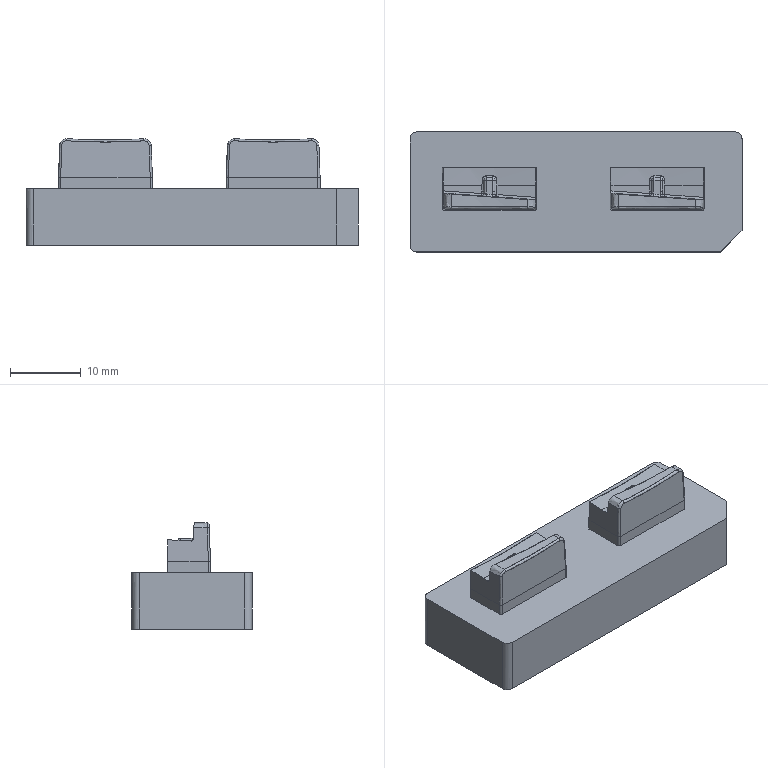NC program | PowerMill | posted with a generic post | part box 47 x 17 x 15.061 mm
Lines 3610 to 4591 of 128250:
N3707 M6
N3708 S18000 M03
N3709 G00 G90 X0.0 Y0.0
N3710 G43 Z9.8009 H2
N3711
N3712 G05 P10000 R4
N3713 X-10.5099 Y2.0173
N3714 Z0.6643
N3715 G01 Z-0.5357 F3600.0
N3716 X-10.5211 Y1.9983 F6000.0
N3717 G03 X-10.4511 Y1.7272 I0.1706 J-0.1005
N3718 G01 X-9.1254 Y0.9453
N3719 X-6.0495 Y0.7321
N3720 X-5.8566 Y0.7074
N3721 X-5.3686 Y0.551
N3722 X-4.9156 Y0.244
N3723 X-4.5365 Y-0.244
N3724 X-4.3539 Y-0.7321
N3725 X-4.3118 Y-1.2201
N3726 X-4.3123 Y-2.1962
N3727 X-4.3929 Y-2.6843
N3728 X-4.5968 Y-3.1723
N3729 X-4.8805 Y-3.5483
N3730 X-5.3686 Y-3.9453
N3731 X-5.8411 Y-4.1484
N3732 X-6.3447 Y-4.2605
N3733 X-6.8327 Y-4.2847
N3734 X-7.3208 Y-4.273
N3735 X-9.273 Y-4.208
N3736 X-12.2013 Y-4.1485
N3737 X-12.2049
N3738 X-14.6416 Y-4.1885
N3739 X-14.644 Y-4.1886
N3740 X-16.1057 Y-4.2487
N3741 X-18.0579 Y-4.2761
N3742 X-18.546 Y-4.1942
N3743 X-19.0341 Y-4.0252
N3744 X-19.5221 Y-3.6941
N3745 X-19.9587 Y-3.1723
N3746 X-20.1576 Y-2.6843
N3747 X-20.2386 Y-2.1962
N3748 X-20.2423 Y-0.244
N3749 X-20.1671 Y0.244
N3750 X-19.9431 Y0.7321
N3751 X-19.5221 Y1.1919
N3752 X-19.0341 Y1.4666
N3753 X-18.546 Y1.5792
N3754 X-18.0579 Y1.5706
N3755 X-12.2013 Y1.1586
N3756 X-9.1254 Y0.9453
N3757 X-10.5069 Y2.0243 Z-0.7325
N3758 X-10.518 Y2.0053
N3759 G03 X-10.4482 Y1.7341 I0.1704 J-0.1007
N3760 G01 X-9.1249 Y0.9526
N3761 X-5.8566 Y0.7239
N3762 X-5.3686 Y0.6242
N3763 X-4.8805 Y0.3679
N3764 X-4.7296 Y0.244
N3765 X-4.3925 Y-0.163
N3766 X-4.1622 Y-0.7321
N3767 X-4.1172 Y-1.2201
N3768 X-4.1136 Y-2.1962
N3769 X-4.1916 Y-2.6843
N3770 X-4.3831 Y-3.1723
N3771 X-4.7574 Y-3.6604
N3772 X-4.8805 Y-3.7751
N3773 X-5.3686 Y-4.0788
N3774 X-5.5235 Y-4.1484
N3775 X-5.8566 Y-4.2484
N3776 X-6.3447 Y-4.3063
N3777 X-18.0579 Y-4.3078
N3778 X-18.546 Y-4.2719
N3779 X-19.0229 Y-4.1484
N3780 X-19.5221 Y-3.8849
N3781 X-19.7884 Y-3.6604
N3782 X-20.0102 Y-3.4027
N3783 X-20.1648 Y-3.1723
N3784 X-20.3576 Y-2.6843
N3785 X-20.4355 Y-2.1962
N3786 X-20.4359 Y-0.244
N3787 X-20.3657 Y0.244
N3788 X-20.1506 Y0.7321
N3789 X-20.0102 Y0.9255
N3790 X-19.7071 Y1.2201
N3791 X-19.5221 Y1.3449
N3792 X-19.0341 Y1.5483
N3793 X-18.546 Y1.6072
N3794 X-18.0579 Y1.5775
N3795 X-9.1249 Y0.9526
N3796 X-10.5058 Y2.0311 Z-0.9292
N3797 X-10.517 Y2.0121
N3798 G03 X-10.4472 Y1.741 I0.1705 J-0.1007
N3799 G01 X-9.1244 Y0.9598
N3800 X-5.8566 Y0.7313
N3801 X-5.3686 Y0.6596
N3802 X-4.8805 Y0.4454
N3803 X-4.6133 Y0.244
N3804 X-4.3925 Y0.0053
N3805 X-4.2288 Y-0.244
N3806 X-4.044 Y-0.7321
N3807 X-3.9988 Y-1.2201
N3808 X-3.9973 Y-2.1962
N3809 X-4.0681 Y-2.6843
N3810 X-4.2578 Y-3.1723
N3811 X-4.3925 Y-3.3813
N3812 X-4.6196 Y-3.6604
N3813 X-4.8805 Y-3.8839
N3814 X-5.3533 Y-4.1484
N3815 X-5.8566 Y-4.2818
N3816 X-6.3447 Y-4.314
N3817 X-18.0579 Y-4.3147
N3818 X-18.546 Y-4.3034
N3819 X-19.0341 Y-4.207
N3820 X-19.1947 Y-4.1484
N3821 X-19.5221 Y-3.9769
N3822 X-19.9283 Y-3.6604
N3823 X-20.292 Y-3.1723
N3824 X-20.4814 Y-2.6843
N3825 X-20.5525 Y-2.1962
N3826 X-20.5498 Y-0.244
N3827 X-20.4982 Y0.188
N3828 X-20.2732 Y0.7321
N3829 X-20.0102 Y1.0661
N3830 X-19.8396 Y1.2201
N3831 X-19.5221 Y1.4225
N3832 X-19.0341 Y1.5882
N3833 X-18.546 Y1.6185
N3834 X-9.1244 Y0.9598
N3835 X-10.5054 Y2.0379 Z-1.126
N3836 X-10.5166 Y2.019
N3837 G03 X-10.4468 Y1.7478 I0.1705 J-0.1007
N3838 G01 X-9.1239 Y0.9665
N3839 X-5.7711 Y0.7321
N3840 X-5.3686 Y0.6787
N3841 X-4.8805 Y0.4875
N3842 X-4.5437 Y0.244
N3843 X-4.3925 Y0.0898
N3844 X-4.1598 Y-0.244
N3845 X-3.9762 Y-0.7321
N3846 X-3.9312 Y-1.2201
N3847 X-3.9321 Y-2.1962
N3848 X-4.0012 Y-2.6843
N3849 X-4.1876 Y-3.1723
N3850 X-4.3925 Y-3.4853
N3851 X-4.5414 Y-3.6604
N3852 X-4.8805 Y-3.9396
N3853 X-5.2551 Y-4.1484
N3854 X-5.8566 Y-4.3044
N3855 X-6.3447 Y-4.3216
N3856 X-18.0579 Y-4.3215
N3857 X-18.546 Y-4.3165
N3858 X-19.0341 Y-4.2321
N3859 X-19.2797 Y-4.1484
N3860 X-19.5221 Y-4.0263
N3861 X-19.9879 Y-3.6604
N3862 X-20.3453 Y-3.1723
N3863 X-20.4982 Y-2.8035
N3864 X-20.5981 Y-2.1962
N3865 X-20.5995 Y-0.244
N3866 X-20.5404 Y0.244
N3867 X-20.3329 Y0.7321
N3868 X-20.0102 Y1.1295
N3869 X-19.9062 Y1.2201
N3870 X-19.5221 Y1.4593
N3871 X-19.0341 Y1.6095
N3872 X-18.546 Y1.6254
N3873 X-9.1239 Y0.9665
N3874 X-10.505 Y2.0448 Z-1.3227
N3875 X-10.5161 Y2.0258
N3876 G03 X-10.4463 Y1.7547 I0.1704 J-0.1007
N3877 G01 X-9.1234 Y0.9734
N3878 X-5.6728 Y0.7321
N3879 X-5.3686 Y0.6902
N3880 X-4.8805 Y0.5058
N3881 X-4.5137 Y0.244
N3882 X-4.3925 Y0.1227
N3883 X-4.1322 Y-0.244
N3884 X-3.9486 Y-0.7321
N3885 X-3.9044 Y-1.0772
N3886 X-3.9058 Y-2.1962
N3887 X-3.9737 Y-2.6843
N3888 X-4.1591 Y-3.1723
N3889 X-4.3925 Y-3.525
N3890 X-4.5097 Y-3.6604
N3891 X-4.8805 Y-3.9683
N3892 X-5.2114 Y-4.1484
N3893 X-5.3686 Y-4.2086
N3894 X-5.8566 Y-4.3145
N3895 X-6.3447 Y-4.3285
N3896 X-18.546 Y-4.3251
N3897 X-19.0341 Y-4.2421
N3898 X-19.3017 Y-4.1484
N3899 X-19.5221 Y-4.0377
N3900 X-20.0027 Y-3.6604
N3901 X-20.3558 Y-3.1723
N3902 X-20.4982 Y-2.8311
N3903 X-20.6065 Y-2.1962
N3904 X-20.6099 Y-0.244
N3905 X-20.5493 Y0.244
N3906 X-20.4982 Y0.4071
N3907 X-20.344 Y0.7321
N3908 X-20.0102 Y1.1436
N3909 X-19.8824 Y1.2335
N3910 X-19.7504 Y1.3172
N3911 X-19.5221 Y1.4698
N3912 X-19.0341 Y1.6179
N3913 X-18.546 Y1.6323
N3914 X-9.1234 Y0.9734
N3915 X-10.5053 Y2.0517 Z-1.5194
N3916 X-10.5165 Y2.0327
N3917 G03 X-10.4467 Y1.7616 I0.1705 J-0.1007
N3918 G01 X-9.123 Y0.9797
N3919 X-5.5845 Y0.7321
N3920 X-5.3686 Y0.6981
N3921 X-4.8805 Y0.5177
N3922 X-4.4972 Y0.244
N3923 X-4.3925 Y0.1392
N3924 X-4.1193 Y-0.244
N3925 X-3.9396 Y-0.7321
N3926 X-3.9044 Y-0.9595
N3927 X-3.8984 Y-2.1962
N3928 X-3.9708 Y-2.6843
N3929 X-4.146 Y-3.1723
N3930 X-4.3925 Y-3.5358
N3931 X-4.4548 Y-3.5946
N3932 X-4.5098 Y-3.6604
N3933 X-4.6988 Y-3.8161
N3934 X-4.8805 Y-3.9804
N3935 X-5.1912 Y-4.1484
N3936 X-5.3686 Y-4.2155
N3937 X-5.8566 Y-4.3234
N3938 X-6.3447 Y-4.3353
N3939 X-18.546 Y-4.3322
N3940 X-19.0341 Y-4.2503
N3941 X-19.3238 Y-4.1484
N3942 X-19.5221 Y-4.0484
N3943 X-20.0102 Y-3.666
N3944 X-20.366 Y-3.1723
N3945 X-20.4285 Y-3.0003
N3946 X-20.4982 Y-2.831
N3947 X-20.5034 Y-2.8005
N3948 X-20.5097 Y-2.7834
N3949 X-20.5463 Y-2.6843
N3950 X-20.6138 Y-2.1962
N3951 X-20.6168 Y-0.244
N3952 X-20.5582 Y0.244
N3953 X-20.4982 Y0.4332
N3954 X-20.3552 Y0.7321
N3955 X-20.0102 Y1.1571
N3956 X-19.5221 Y1.4803
N3957 X-19.0341 Y1.6263
N3958 X-18.546 Y1.6392
N3959 X-9.123 Y0.9797
N3960 X-10.5039 Y2.0585 Z-1.7162
N3961 X-10.5151 Y2.0395
N3962 G03 X-10.4453 Y1.7683 I0.1705 J-0.1007
N3963 G01 X-9.1225 Y0.9871
N3964 X-6.3447 Y0.7929
N3965 X-5.9649 Y0.7588
N3966 X-5.5845 Y0.732
N3967 X-5.4841 Y0.7162
N3968 X-5.4775 Y0.7156
N3969 X-5.3686 Y0.7059
N3970 X-4.8805 Y0.5277
N3971 X-4.4836 Y0.244
N3972 X-4.3925 Y0.1529
N3973 X-4.1091 Y-0.244
N3974 X-3.931 Y-0.7321
N3975 X-3.9044 Y-0.8892
N3976 Y-0.9698
N3977 X-3.8985 Y-2.1962
N3978 X-3.9044 Y-2.2364
N3979 Y-2.3937
N3980 X-3.9621 Y-2.6843
N3981 X-4.1358 Y-3.1723
N3982 X-4.3925 Y-3.5503
N3983 X-4.4941 Y-3.6422
N3984 X-4.5098 Y-3.6603
N3985 X-4.5632 Y-3.7047
N3986 X-4.8805 Y-3.9916
N3987 X-5.1686 Y-4.1484
N3988 X-5.3686 Y-4.2225
N3989 X-5.8566 Y-4.331
N3990 X-6.3447 Y-4.3422
N3991 X-18.546 Y-4.3392
N3992 X-19.0341 Y-4.2584
N3993 X-19.3459 Y-4.1484
N3994 X-19.5221 Y-4.059
N3995 X-20.0102 Y-3.6792
N3996 X-20.3762 Y-3.1723
N3997 X-20.5546 Y-2.6843
N3998 X-20.6207 Y-2.1962
N3999 X-20.6236 Y-0.244
N4000 X-20.567 Y0.244
N4001 X-20.4982 Y0.4594
N4002 X-20.3664 Y0.7321
N4003 X-20.0102 Y1.1707
N4004 X-19.5221 Y1.4908
N4005 X-19.0341 Y1.6347
N4006 X-18.546 Y1.6461
N4007 X-9.1225 Y0.9871
N4008 X-10.5035 Y2.0653 Z-1.9129
N4009 X-10.5146 Y2.0464
N4010 G03 X-10.4448 Y1.7752 I0.1704 J-0.1007
N4011 G01 X-9.122 Y0.994
N4012 X-5.8566 Y0.7656
N4013 X-5.4698 Y0.7321
N4014 X-5.3984 Y0.7085
N4015 X-5.3686 Y0.7059
N4016 X-5.1655 Y0.6317
N4017 X-5.1625 Y0.6307
N4018 X-4.8805 Y0.5377
N4019 X-4.47 Y0.244
N4020 X-4.3649 Y0.114
N4021 X-4.2677 Y-0.0219
N4022 X-4.0988 Y-0.244
N4023 X-3.9228 Y-0.7321
N4024 X-3.917 Y-0.811
N4025 X-3.9045 Y-0.8892
N4026 Y-0.9568
N4027 X-3.883 Y-1.2201
N4028 X-3.8846 Y-2.1962
N4029 X-3.9044 Y-2.4516
N4030 X-3.9535 Y-2.6843
N4031 X-4.1256 Y-3.1723
N4032 X-4.3925 Y-3.5648
N4033 X-4.8805 Y-4.0027
N4034 X-5.146 Y-4.1484
N4035 X-5.3686 Y-4.2312
N4036 X-5.8566 Y-4.3386
N4037 X-6.3447 Y-4.3491
N4038 X-18.546 Y-4.3462
N4039 X-19.0341 Y-4.2666
N4040 X-19.3679 Y-4.1484
N4041 X-19.5221 Y-4.0697
N4042 X-20.0102 Y-3.6924
N4043 X-20.3864 Y-3.1723
N4044 X-20.5629 Y-2.6843
N4045 X-20.6276 Y-2.1962
N4046 X-20.6305 Y-0.244
N4047 X-20.5759 Y0.244
N4048 X-20.4982 Y0.4839
N4049 X-20.3776 Y0.7321
N4050 X-20.0102 Y1.1843
N4051 X-19.5221 Y1.5013
N4052 X-19.0341 Y1.6431
N4053 X-18.546 Y1.6529
N4054 X-9.122 Y0.994
N4055 X-10.5197 Y2.082 Z-2.1097
N4056 X-10.5309 Y2.0631
N4057 G03 X-10.4611 Y1.7919 I0.1705 J-0.1007
N4058 G01 X-9.1215 Y1.0008
N4059 X-5.8566 Y0.7725
N4060 X-5.424 Y0.7321
N4061 X-4.8805 Y0.5477
N4062 X-4.4563 Y0.244
N4063 X-4.0886 Y-0.244
N4064 X-3.9146 Y-0.7321
N4065 X-3.8761 Y-1.2201
N4066 X-3.8778 Y-2.1962
N4067 X-3.9044 Y-2.5017
N4068 X-3.9448 Y-2.6843
N4069 X-4.1154 Y-3.1723
N4070 X-4.3925 Y-3.5792
N4071 X-4.8805 Y-4.0139
N4072 X-5.1233 Y-4.1484
N4073 X-5.3686 Y-4.24
N4074 X-5.8566 Y-4.3462
N4075 X-6.222 Y-4.3464
N4076 X-6.224
N4077 X-6.3447 Y-4.349
N4078 X-9.6022 Y-4.3483
N4079 X-18.546 Y-4.3532
N4080 X-19.0341 Y-4.2747
N4081 X-19.1998 Y-4.2083
N4082 X-19.3679 Y-4.1484
N4083 X-19.4434 Y-4.1108
N4084 X-19.5221 Y-4.0804
N4085 X-20.0102 Y-3.7057
N4086 X-20.3966 Y-3.1723
N4087 X-20.5712 Y-2.6843
N4088 X-20.6344 Y-2.1962
N4089 X-20.6374 Y-0.244
N4090 X-20.5848 Y0.244
N4091 X-20.4982 Y0.5083
N4092 X-20.3888 Y0.7321
N4093 X-20.0102 Y1.1979
N4094 X-19.5221 Y1.5118
N4095 X-19.0341 Y1.6515
N4096 X-18.546 Y1.6598
N4097 X-9.1215 Y1.0008
N4098 X-10.5127 Y2.0851 Z-2.3064
N4099 X-10.5239 Y2.0661
N4100 G03 X-10.4541 Y1.7949 I0.1705 J-0.1007
N4101 G01 X-9.121 Y1.0077
N4102 X-5.8566 Y0.7794
N4103 X-5.3822 Y0.7321
N4104 X-4.8805 Y0.5577
N4105 X-4.4427 Y0.244
N4106 X-4.0784 Y-0.244
N4107 X-3.9064 Y-0.7321
N4108 X-3.8693 Y-1.2201
N4109 X-3.8709 Y-2.1962
N4110 X-3.9044 Y-2.5467
N4111 X-3.9366 Y-2.647
N4112 X-3.9449 Y-2.6843
N4113 X-3.9904 Y-2.8145
N4114 X-3.9912 Y-2.8169
N4115 X-4.1053 Y-3.1723
N4116 X-4.3925 Y-3.5937
N4117 X-4.8805 Y-4.0251
N4118 X-5.1023 Y-4.1484
N4119 X-5.3686 Y-4.2487
N4120 X-5.8566 Y-4.3536
N4121 X-18.546 Y-4.3602
N4122 X-19.0341 Y-4.2829
N4123 X-19.5221 Y-4.0911
N4124 X-20.0102 Y-3.7189
N4125 X-20.4068 Y-3.1723
N4126 X-20.5795 Y-2.6843
N4127 X-20.6413 Y-2.1962
N4128 X-20.6443 Y-0.244
N4129 X-20.5937 Y0.244
N4130 X-20.4982 Y0.5328
N4131 X-20.4 Y0.7321
N4132 X-20.0102 Y1.2114
N4133 X-19.5221 Y1.5223
N4134 X-19.0341 Y1.66
N4135 X-18.546 Y1.6667
N4136 X-13.1774 Y1.2913
N4137 X-12.6894 Y1.2725
N4138 X-11.2252 Y1.1548
N4139 X-9.121 Y1.0077
N4140 X-10.5866 Y2.1358 Z-2.5031
N4141 X-10.5978 Y2.1169
N4142 G03 X-10.528 Y1.8457 I0.1705 J-0.1007
N4143 G01 X-9.1206 Y1.0145
N4144 X-5.8566 Y0.7863
N4145 X-5.3686 Y0.7373
N4146 X-4.8805 Y0.5677
N4147 X-4.4291 Y0.244
N4148 X-4.0681 Y-0.244
N4149 X-3.9044 Y-0.7028
N4150 X-3.8624 Y-1.2201
N4151 X-3.864 Y-2.1962
N4152 X-3.9044 Y-2.5877
N4153 X-4.0951 Y-3.1723
N4154 X-4.3925 Y-3.6082
N4155 X-4.8805 Y-4.0363
N4156 X-5.0813 Y-4.1484
N4157 X-5.3686 Y-4.2575
N4158 X-5.8566 Y-4.361
N4159 X-18.546 Y-4.3672
N4160 X-19.0341 Y-4.291
N4161 X-19.5221 Y-4.1017
N4162 X-20.0102 Y-3.7316
N4163 X-20.417 Y-3.1723
N4164 X-20.5877 Y-2.6843
N4165 X-20.6482 Y-2.1962
N4166 X-20.6511 Y-0.244
N4167 X-20.6026 Y0.244
N4168 X-20.4982 Y0.5572
N4169 X-20.4112 Y0.7321
N4170 X-20.0165 Y1.2201
N4171 X-19.5221 Y1.5328
N4172 X-19.0341 Y1.6702
N4173 X-18.546 Y1.6736
N4174 X-13.4288 Y1.3158
N4175 X-13.1774 Y1.383
N4176 X-12.6894 Y1.4397
N4177 X-11.7133 Y1.3738
N4178 X-11.2252 Y1.2827
N4179 X-10.7372 Y1.1276
N4180 X-10.7137 Y1.1259
N4181 X-10.7133
N4182 X-9.1206 Y1.0145
N4183 X-7.0709 Y1.8923 Z-2.6984
N4184 X-7.0821 Y1.8733
N4185 G03 X-7.0126 Y1.6021 I0.1703 J-0.1008
N4186 G01 X-5.6107 Y0.7721
N4187 X-5.3686 Y0.7549
N4188 X-4.8805 Y0.5875
N4189 X-4.4056 Y0.244
N4190 X-4.0531 Y-0.244
N4191 X-3.9044 Y-0.6554
N4192 X-3.8556 Y-1.2201
N4193 X-3.8572 Y-2.1962
N4194 X-3.9044 Y-2.6243
N4195 X-4.085 Y-3.1723
N4196 X-4.3925 Y-3.6225
N4197 X-4.8805 Y-4.0473
N4198 X-5.0604 Y-4.1484
N4199 X-5.3686 Y-4.2662
N4200 X-5.8566 Y-4.3682
N4201 X-6.3447 Y-4.3765
N4202 X-18.546 Y-4.3742
N4203 X-19.0341 Y-4.2991
N4204 X-19.5221 Y-4.1123
N4205 X-19.8242 Y-3.8725
N4206 X-20.0101 Y-3.7316
N4207 X-20.0251 Y-3.7148
N4208 X-20.0419 Y-3.6998
N4209 X-20.0916 Y-3.6604
N4210 X-20.4272 Y-3.1723
N4211 X-20.596 Y-2.6843
N4212 X-20.655 Y-2.1962
N4213 X-20.6579 Y-0.244
N4214 X-20.6154 Y0.244
N4215 X-20.4995 Y0.5531
N4216 X-20.4982 Y0.5572
N4217 X-20.4967 Y0.5608
N4218 X-20.4953 Y0.5645
N4219 X-20.4324 Y0.7321
N4220 X-20.0497 Y1.2201
N4221 X-19.5221 Y1.5608
N4222 X-19.0341 Y1.694
N4223 X-18.8683 Y1.7082
N4224 X-15.0658 Y1.4374
N4225 G03 X-14.8516 Y1.6373 I0.0142 J0.1995
N4226 G01 X-14.8517 Y1.7082
N4227 X-14.7863 Y2.1962
N4228 X-14.5904 Y2.6843
N4229 X-14.231 Y3.1723
N4230 X-13.6655 Y3.5832
N4231 X-13.4923 Y3.6604
N4232 X-13.1774 Y3.7505
N4233 X-12.6894 Y3.8054
N4234 X-11.7133 Y3.804
N4235 X-11.2252 Y3.7289
N4236 X-11.0156 Y3.6604
N4237 X-10.7372 Y3.5243
N4238 X-10.276 Y3.1723
N4239 X-9.91 Y2.6843
N4240 X-9.7611 Y2.3294
N4241 X-9.6543 Y1.7082
N4242 X-9.659 Y1.2479
N4243 G03 X-9.4732 Y1.0464 I0.2 J-0.002
N4244 G01 X-5.6107 Y0.7721
N4245 X-2.8721 Y2.2454 Z-2.8937
N4246 X-2.8918 Y2.2553
N4247 G03 X-3.1574 Y2.1668 I-0.0886 J-0.1771
N4248 G01 X-3.8551 Y0.7719
N4249 X-3.8552 Y0.244
N4250 X-3.9044 Y-0.0613
N4251 X-3.9457 Y-0.1931
N4252 X-3.954 Y-0.2306
N4253 X-3.9525 Y-0.269
N4254 X-3.9504 Y-0.2947
N4255 X-3.8568 Y-0.7321
N4256 X-3.8503 Y-2.1962
N4257 X-3.9044 Y-2.66
N4258 X-4.0749 Y-3.1723
N4259 X-4.3925 Y-3.6369
N4260 X-4.8805 Y-4.0584
N4261 X-5.0396 Y-4.1484
N4262 X-5.3686 Y-4.2748
N4263 X-5.8566 Y-4.3755
N4264 X-6.3447 Y-4.3833
N4265 X-18.546 Y-4.3812
N4266 X-19.0341 Y-4.3072
N4267 X-19.4723 Y-4.1484
N4268 X-19.5218 Y-4.1124
N4269 X-19.5221 Y-4.1123
N4270 X-19.5235 Y-4.1112
N4271 X-20.0102 Y-3.7563
N4272 X-20.1042 Y-3.6604
N4273 X-20.4373 Y-3.1723
N4274 X-20.6042 Y-2.6843
N4275 X-20.6619 Y-2.1962
N4276 X-20.6587 Y3.6604
N4277 X-20.537 Y4.1484
N4278 X-20.2497 Y4.6365
N4279 X-20.0102 Y4.8798
N4280 X-19.6442 Y5.1246
N4281 X-19.0341 Y5.3112
N4282 X-16.1057 Y5.326
N4283 X-15.6177 Y5.3015
N4284 X-15.0448 Y5.1246
N4285 X-14.6416 Y4.8418
N4286 X-14.4313 Y4.6365
N4287 X-14.1367 Y4.1484
N4288 X-14.0358 Y3.7474
N4289 G03 X-13.7397 Y3.6242 I0.194 J0.0488
N4290 G01 X-13.6655 Y3.6683
N4291 X-13.1774 Y3.8309
N4292 X-12.6894 Y3.8848
N4293 X-11.7133 Y3.8832
N4294 X-11.2252 Y3.811
N4295 X-10.8296 Y3.6604
N4296 X-10.7082 Y3.5857
N4297 G03 X-10.4075 Y3.7156 I0.1048 J0.1704
N4298 G01 X-10.318 Y4.1484
N4299 X-10.2491 Y4.2237
N4300 X-10.0407 Y4.6365
N4301 X-9.7611 Y4.8786
N4302 X-9.4105 Y5.1246
N4303 X-8.7849 Y5.3007
N4304 X-8.2969 Y5.326
N4305 X-5.8566
N4306 X-5.3686 Y5.2919
N4307 X-4.8695 Y5.1246
N4308 X-4.3925 Y4.7807
N4309 X-4.2619 Y4.6365
N4310 X-3.9751 Y4.1484
N4311 X-3.9044 Y3.9336
N4312 X-3.8548 Y3.6604
N4313 X-3.8551 Y0.7719
N4314 X-2.8652 Y2.2224 Z-3.089
N4315 X-2.8849 Y2.2323
N4316 G03 X-3.1506 Y2.1441 I-0.0888 J-0.177
N4317 G01 X-3.8392 Y0.7718
N4318 X-3.8435 Y-2.1962
N4319 X-3.9018 Y-2.6843
N4320 X-4.0648 Y-3.1723
N4321 X-4.3925 Y-3.6512
N4322 X-4.8805 Y-4.0695
N4323 X-5.0187 Y-4.1484
N4324 X-5.3686 Y-4.2835
N4325 X-5.8566 Y-4.3828
N4326 X-6.3447 Y-4.3902
N4327 X-18.546 Y-4.3881
N4328 X-19.0341 Y-4.3153
N4329 X-19.493 Y-4.1484
N4330 X-20.0102 Y-3.7687
N4331 X-20.1168 Y-3.6604
N4332 X-20.4474 Y-3.1723
N4333 X-20.6124 Y-2.6843
N4334 X-20.6687 Y-2.1962
N4335 X-20.6764 Y3.1723
N4336 X-20.6655 Y3.6604
N4337 X-20.5438 Y4.1484
N4338 X-20.2571 Y4.6365
N4339 X-20.0102 Y4.8872
N4340 X-19.6511 Y5.1246
N4341 X-19.5221 Y5.1819
N4342 X-19.0341 Y5.3121
N4343 X-18.546 Y5.326
N4344 X-5.8566
N4345 X-5.3686 Y5.2943
N4346 X-4.8611 Y5.1246
N4347 X-4.3925 Y4.7872
N4348 X-4.2551 Y4.6365
N4349 X-3.9683 Y4.1484
N4350 X-3.9044 Y3.9587
N4351 X-3.8466 Y3.6604
N4352 X-3.8358 Y3.1723
N4353 X-3.8392 Y0.7718
N4354 X-2.8584 Y2.2224 Z-3.2843
N4355 X-2.878 Y2.2323
N4356 G03 X-3.1438 Y2.1441 I-0.0888 J-0.177
N4357 G01 X-3.8324 Y0.7718
N4358 X-3.8367 Y-2.1962
N4359 X-3.8934 Y-2.6843
N4360 X-4.0547 Y-3.1723
N4361 X-4.3878 Y-3.6604
N4362 X-4.8805 Y-4.0806
N4363 X-4.9986 Y-4.1484
N4364 X-5.3686 Y-4.2922
N4365 X-5.8566 Y-4.3901
N4366 X-6.3447 Y-4.397
N4367 X-18.546 Y-4.3951
N4368 X-19.0341 Y-4.3234
N4369 X-19.5136 Y-4.1484
N4370 X-20.0102 Y-3.781
N4371 X-20.1294 Y-3.6604
N4372 X-20.4576 Y-3.1723
N4373 X-20.6206 Y-2.6843
N4374 X-20.6755 Y-2.1962
N4375 X-20.6832 Y3.1723
N4376 X-20.6724 Y3.6604
N4377 X-20.5507 Y4.1484
N4378 X-20.2639 Y4.6365
N4379 X-20.0102 Y4.8928
N4380 X-19.6579 Y5.1246
N4381 X-19.5221 Y5.1866
N4382 X-19.0341 Y5.3129
N4383 X-18.546 Y5.326
N4384 X-5.8566
N4385 X-5.3686 Y5.2967
N4386 X-4.8805 Y5.1372
N4387 X-4.8764 Y5.1342
N4388 X-4.8688 Y5.1292
N4389 X-4.8611 Y5.1245
N4390 X-4.7975 Y5.0787
N4391 X-4.3925 Y4.7936
N4392 X-4.2483 Y4.6365
N4393 X-3.9615 Y4.1484
N4394 X-3.9044 Y3.9827
N4395 X-3.8398 Y3.6604
N4396 X-3.829 Y3.1723
N4397 X-3.8324 Y0.7718
N4398 X-2.8515 Y2.2225 Z-3.4796
N4399 X-2.8712 Y2.2323
N4400 G03 X-3.137 Y2.1442 I-0.0888 J-0.1769
N4401 G01 X-3.8256 Y0.7718
N4402 X-3.8298 Y-2.1962
N4403 X-3.885 Y-2.6843
N4404 X-4.0446 Y-3.1723
N4405 X-4.3749 Y-3.6604
N4406 X-4.8805 Y-4.0917
N4407 X-4.9793 Y-4.1484
N4408 X-5.3686 Y-4.3009
N4409 X-5.8566 Y-4.3973
N4410 X-6.3447 Y-4.4038
N4411 X-18.546 Y-4.4021
N4412 X-19.0341 Y-4.3315
N4413 X-19.5221 Y-4.1544
N4414 X-20.0102 Y-3.7934
N4415 X-20.142 Y-3.6604
N4416 X-20.4677 Y-3.1723
N4417 X-20.6289 Y-2.6843
N4418 X-20.6824 Y-2.1962
N4419 X-20.69 Y3.1723
N4420 X-20.6792 Y3.6604
N4421 X-20.5575 Y4.1484
N4422 X-20.4982 Y4.2804
N4423 X-20.2707 Y4.6365
N4424 X-20.0102 Y4.8981
N4425 X-19.6647 Y5.1246
N4426 X-19.5221 Y5.1893
N4427 X-19.0341 Y5.3137
N4428 X-18.546 Y5.326
N4429 X-5.8566
N4430 X-5.3686 Y5.2979
N4431 X-4.8805 Y5.1409
N4432 X-4.3925 Y4.8
N4433 X-4.2415 Y4.6365
N4434 X-3.9547 Y4.1484
N4435 X-3.9046 Y3.9741
N4436 X-3.8669 Y3.7966
N4437 X-3.833 Y3.6604
N4438 X-3.8222 Y3.1723
N4439 X-3.8256 Y0.7718
N4440 X-2.8447 Y2.2225 Z-3.6749
N4441 X-2.8644 Y2.2323
N4442 G03 X-3.1301 Y2.1442 I-0.0888 J-0.1769
N4443 G01 X-3.8188 Y0.7718
N4444 X-3.823 Y-2.1962
N4445 X-3.8767 Y-2.6843
N4446 X-4.0345 Y-3.1723
N4447 X-4.362 Y-3.6604
N4448 X-4.6626 Y-3.9057
N4449 X-4.8806 Y-4.0916
N4450 X-4.9226 Y-4.1168
N4451 X-4.96 Y-4.1484
N4452 X-5.3686 Y-4.3095
N4453 X-5.8566 Y-4.4046
N4454 X-6.3447 Y-4.4106
N4455 X-18.546 Y-4.409
N4456 X-19.0341 Y-4.3396
N4457 X-19.5221 Y-4.1646
N4458 X-20.0102 Y-3.8057
N4459 X-20.1546 Y-3.6604
N4460 X-20.4778 Y-3.1723
N4461 X-20.6371 Y-2.6843
N4462 X-20.6892 Y-2.1962
N4463 X-20.6968 Y3.1723
N4464 X-20.686 Y3.6604
N4465 X-20.5643 Y4.1484
N4466 X-20.4982 Y4.2943
N4467 X-20.2775 Y4.6365
N4468 X-20.0102 Y4.9035
N4469 X-19.6715 Y5.1246
N4470 X-19.5221 Y5.1921
N4471 X-19.0341 Y5.3145
N4472 X-18.546 Y5.326
N4473 X-5.8566
N4474 X-5.3686 Y5.299
N4475 X-4.8805 Y5.1441
N4476 X-4.3925 Y4.8064
N4477 X-4.2346 Y4.6365
N4478 X-3.9479 Y4.1484
N4479 X-3.9118 Y4.0038
N4480 X-3.9045 Y3.9827
N4481 X-3.8963 Y3.9416
N4482 X-3.8952 Y3.9372
N4483 X-3.8262 Y3.6604
N4484 X-3.8153 Y3.1723
N4485 X-3.8188 Y0.7718
N4486 X-2.8435 Y2.2112 Z-3.8701
N4487 X-2.8632 Y2.2211
N4488 G03 X-3.129 Y2.1329 I-0.0888 J-0.177
N4489 G01 X-3.8119 Y0.7718
N4490 X-3.8162 Y-2.1962
N4491 X-3.8683 Y-2.6843
N4492 X-4.0244 Y-3.1723
N4493 X-4.3491 Y-3.6604
N4494 X-4.9407 Y-4.1484
N4495 X-5.3686 Y-4.3182
N4496 X-5.8566 Y-4.4119
N4497 X-6.3447 Y-4.4174
N4498 X-18.546 Y-4.416
N4499 X-19.0341 Y-4.3477
N4500 X-19.5221 Y-4.1748
N4501 X-20.0102 Y-3.8181
N4502 X-20.1672 Y-3.6604
N4503 X-20.488 Y-3.1723
N4504 X-20.6453 Y-2.6843
N4505 X-20.696 Y-2.1962
N4506 X-20.7036 Y3.1723
N4507 X-20.6928 Y3.6604
N4508 X-20.5711 Y4.1484
N4509 X-20.4982 Y4.3083
N4510 X-20.2843 Y4.6365
N4511 X-20.0102 Y4.9088
N4512 X-19.6784 Y5.1246
N4513 X-19.5221 Y5.1948
N4514 X-19.0341 Y5.3153
N4515 X-18.546 Y5.326
N4516 X-5.8566
N4517 X-5.3686 Y5.3002
N4518 X-4.8805 Y5.1474
N4519 X-4.3925 Y4.8128
N4520 X-4.2278 Y4.6365
N4521 X-3.941 Y4.1484
N4522 X-3.8193 Y3.6604
N4523 X-3.8085 Y3.1723
N4524 X-3.8119 Y0.7718
N4525 X-2.8434 Y2.198 Z-4.0654
N4526 X-2.863 Y2.2078
N4527 G03 X-3.1288 Y2.1196 I-0.0888 J-0.177
N4528 G01 X-3.8051 Y0.7718
N4529 X-3.8093 Y-2.1962
N4530 X-3.8599 Y-2.6843
N4531 X-4.0143 Y-3.1723
N4532 X-4.3362 Y-3.6604
N4533 X-4.9214 Y-4.1484
N4534 X-5.3686 Y-4.3269
N4535 X-5.8566 Y-4.4192
N4536 X-6.3447 Y-4.4243
N4537 X-18.546 Y-4.423
N4538 X-19.0341 Y-4.3563
N4539 X-19.5221 Y-4.1849
N4540 X-20.0102 Y-3.8304
N4541 X-20.1798 Y-3.6604
N4542 X-20.4981 Y-3.1723
N4543 X-20.6535 Y-2.6843
N4544 X-20.7028 Y-2.1962
N4545 X-20.7105 Y3.1723
N4546 X-20.6996 Y3.6604
N4547 X-20.5779 Y4.1484
N4548 X-20.4982 Y4.322
N4549 X-20.2911 Y4.6365
N4550 X-20.0102 Y4.9142
N4551 X-19.6852 Y5.1246
N4552 X-19.5221 Y5.1975
N4553 X-19.0341 Y5.316
N4554 X-18.546 Y5.326
N4555 X-5.8566
N4556 X-5.3686 Y5.3013
N4557 X-4.8805 Y5.1506
N4558 X-4.3925 Y4.8193
N4559 X-4.221 Y4.6365
N4560 X-3.9342 Y4.1484
N4561 X-3.8125 Y3.6604
N4562 X-3.8017 Y3.1723
N4563 X-3.8051 Y0.7718
N4564 X-2.8365 Y2.198 Z-4.2607
N4565 X-2.8562 Y2.2079
N4566 G03 X-3.1219 Y2.1197 I-0.0888 J-0.177
N4567 G01 X-3.7983 Y0.7718
N4568 X-3.8025 Y-2.1962
N4569 X-3.8515 Y-2.6843
N4570 X-4.0042 Y-3.1723
N4571 X-4.3232 Y-3.6604
N4572 X-4.9021 Y-4.1484
N4573 X-5.3686 Y-4.3356
N4574 X-5.8566 Y-4.4264
N4575 X-6.3447 Y-4.4311
N4576 X-18.546 Y-4.4299
N4577 X-19.0341 Y-4.365
N4578 X-19.5221 Y-4.1951
N4579 X-20.0102 Y-3.8436
N4580 X-20.1924 Y-3.6604
N4581 X-20.4982 Y-3.1934
N4582 X-20.6618 Y-2.6843
N4583 X-20.7097 Y-2.1962
N4584 X-20.7173 Y3.1723
N4585 X-20.7065 Y3.6604
N4586 X-20.5847 Y4.1484
N4587 X-20.4982 Y4.3343
N4588 X-20.298 Y4.6365
N4589 X-20.0102 Y4.9196
N4590 X-19.692 Y5.1246
N4591 X-19.5221 Y5.2002
N4592 X-19.0341 Y5.3167
N4593 X-18.546 Y5.326
N4594 X-5.8566
N4595 X-5.3686 Y5.3024
N4596 X-4.8805 Y5.1537
N4597 X-4.3925 Y4.8257
N4598 X-4.2142 Y4.6365
N4599 X-3.9274 Y4.1484
N4600 X-3.8057 Y3.6604
N4601 X-3.7949 Y3.1723
N4602 X-3.7983 Y0.7718
N4603 X-2.8297 Y2.198 Z-4.456
N4604 X-2.8493 Y2.2079
N4605 G03 X-3.1151 Y2.1197 I-0.0888 J-0.177
N4606 G01 X-3.7915 Y0.7718
N4607 X-3.7957 Y-2.1962
N4608 X-3.8432 Y-2.6843
N4609 X-3.9945 Y-3.1723
N4610 X-4.3103 Y-3.6604
N4611 X-4.8829 Y-4.1484
N4612 X-5.3686 Y-4.3443
N4613 X-5.8566 Y-4.4337
N4614 X-6.3447 Y-4.4379
N4615 X-18.546 Y-4.4369
N4616 X-19.0341 Y-4.3737
N4617 X-19.5221 Y-4.2052
N4618 X-19.6291 Y-4.1484
N4619 X-20.0102 Y-3.857
N4620 X-20.205 Y-3.6604
N4621 X-20.4982 Y-3.2146
N4622 X-20.67 Y-2.6843
N4623 X-20.7165 Y-2.1962
N4624 X-20.7241 Y3.1723
N4625 X-20.7133 Y3.6604
N4626 X-20.5916 Y4.1484
N4627 X-20.4982 Y4.3467
N4628 X-20.3048 Y4.6365
N4629 X-20.0102 Y4.9249
N4630 X-19.6988 Y5.1246
N4631 X-19.5221 Y5.2028
N4632 X-19.0341 Y5.3174
N4633 X-18.546 Y5.326
N4634 X-5.8566
N4635 X-5.3686 Y5.3035
N4636 X-4.8805 Y5.1569
N4637 X-4.3925 Y4.8321
N4638 X-4.2074 Y4.6365
N4639 X-3.9206 Y4.1484
N4640 X-3.7989 Y3.6604
N4641 X-3.7881 Y3.1723
N4642 X-3.7915 Y0.7718
N4643 X-2.8228 Y2.1981 Z-4.6513
N4644 X-2.8425 Y2.2079
N4645 G03 X-3.1082 Y2.1198 I-0.0888 J-0.1769
N4646 G01 X-3.7846 Y0.7718
N4647 X-3.7888 Y-2.1962
N4648 X-3.8348 Y-2.6843
N4649 X-3.9847 Y-3.1723
N4650 X-4.2974 Y-3.6604
N4651 X-4.8647 Y-4.1484
N4652 X-5.3686 Y-4.3529
N4653 X-5.8566 Y-4.441
N4654 X-6.3447 Y-4.4447
N4655 X-18.546 Y-4.4438
N4656 X-19.0341 Y-4.3824
N4657 X-19.5221 Y-4.2154
N4658 X-19.6477 Y-4.1484
N4659 X-20.0102 Y-3.8704
N4660 X-20.2176 Y-3.6604
N4661 X-20.4982 Y-3.2359
N4662 X-20.6782 Y-2.6843
N4663 X-20.7233 Y-2.1962
N4664 X-20.7309 Y3.1723
N4665 X-20.7201 Y3.6604
N4666 X-20.5984 Y4.1484
N4667 X-20.4982 Y4.359
N4668 X-20.3116 Y4.6365
N4669 X-20.0102 Y4.9303
N4670 X-19.7056 Y5.1246
N4671 X-19.5221 Y5.2054
N4672 X-19.0341 Y5.318
N4673 X-18.546 Y5.326
N4674 X-5.8566
N4675 X-5.3686 Y5.3046
N4676 X-4.8805 Y5.1599
N4677 X-4.3925 Y4.8385
N4678 X-4.2006 Y4.6365
N4679 X-3.9138 Y4.1484
N4680 X-3.7921 Y3.6604
N4681 X-3.7812 Y3.1723
N4682 X-3.7846 Y0.7718
N4683 X-2.816 Y2.1981 Z-4.8466
N4684 X-2.8356 Y2.208
N4685 G03 X-3.1014 Y2.1198 I-0.0888 J-0.177
N4686 G01 X-3.7778 Y0.7717
N4687 X-3.782 Y-2.1962
N4688 X-3.8264 Y-2.6843